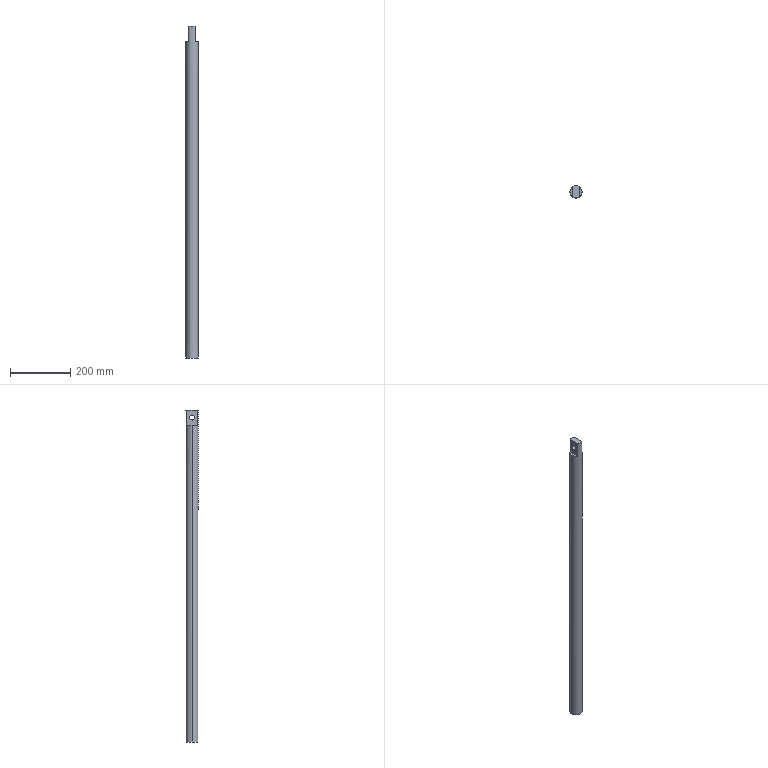Part | SolidWorks | features ICE 2, Extrusion 1 | 1 solid | 10 faces | box 40 x 40 x 1100 mm | volume 1353457 mm3 | plane 6 | cylinder 4 | commonest cylinder face diameters 16.5 x2 40 x2
STEP:
#1=CARTESIAN_POINT('',(10.,0.,1066.75));
#2=VERTEX_POINT('',#1);
#3=CARTESIAN_POINT('',(10.,0.,1083.25));
#4=VERTEX_POINT('',#3);
#5=CARTESIAN_POINT('',(10.,0.,1075.));
#6=DIRECTION('',(-1.,0.,0.));
#7=DIRECTION('',(0.,0.,1.));
#8=AXIS2_PLACEMENT_3D('',#5,#6,#7);
#9=CIRCLE('',#8,8.25);
#10=EDGE_CURVE('',#2,#4,#9,.T.);
#11=ORIENTED_EDGE('',*,*,#10,.F.);
#12=CARTESIAN_POINT('',(-10.,0.,1066.75));
#13=VERTEX_POINT('',#12);
#14=CARTESIAN_POINT('',(20.,0.,1066.75));
#15=DIRECTION('',(-1.,0.,0.));
#16=VECTOR('',#15,1000.);
#17=LINE('',#14,#16);
#18=EDGE_CURVE('',#2,#13,#17,.T.);
#19=ORIENTED_EDGE('',*,*,#18,.T.);
#20=CARTESIAN_POINT('',(-10.,0.,1083.25));
#21=VERTEX_POINT('',#20);
#22=CARTESIAN_POINT('',(-10.,0.,1075.));
#23=DIRECTION('',(1.,0.,0.));
#24=DIRECTION('',(0.,0.,-1.));
#25=AXIS2_PLACEMENT_3D('',#22,#23,#24);
#26=CIRCLE('',#25,8.25);
#27=EDGE_CURVE('',#21,#13,#26,.T.);
#28=ORIENTED_EDGE('',*,*,#27,.F.);
#29=CARTESIAN_POINT('',(20.,0.,1083.25));
#30=DIRECTION('',(-1.,0.,0.));
#31=VECTOR('',#30,1000.);
#32=LINE('',#29,#31);
#33=EDGE_CURVE('',#4,#21,#32,.T.);
#34=ORIENTED_EDGE('',*,*,#33,.F.);
#35=EDGE_LOOP('',(#11,#19,#28,#34));
#36=FACE_OUTER_BOUND('',#35,.T.);
#37=CARTESIAN_POINT('',(20.,0.,1075.));
#38=DIRECTION('',(-1.,0.,0.));
#39=DIRECTION('',(0.,0.,1.));
#40=AXIS2_PLACEMENT_3D('',#37,#38,#39);
#41=CYLINDRICAL_SURFACE('',#40,8.25);
#42=ADVANCED_FACE('',(#36),#41,.F.);
#43=CARTESIAN_POINT('',(10.,17.321,1050.));
#44=VERTEX_POINT('',#43);
#45=CARTESIAN_POINT('',(20.,0.,1050.));
#46=VERTEX_POINT('',#45);
#47=CARTESIAN_POINT('',(0.,0.,1050.));
#48=DIRECTION('',(0.,0.,-1.));
#49=DIRECTION('',(-1.,0.,0.));
#50=AXIS2_PLACEMENT_3D('',#47,#48,#49);
#51=CIRCLE('',#50,20.);
#52=EDGE_CURVE('',#44,#46,#51,.T.);
#53=ORIENTED_EDGE('',*,*,#52,.T.);
#54=CARTESIAN_POINT('',(20.,0.,0.));
#55=VERTEX_POINT('',#54);
#56=CARTESIAN_POINT('',(20.,0.,1100.));
#57=DIRECTION('',(0.,0.,-1.));
#58=VECTOR('',#57,1000.);
#59=LINE('',#56,#58);
#60=EDGE_CURVE('',#46,#55,#59,.T.);
#61=ORIENTED_EDGE('',*,*,#60,.T.);
#62=CARTESIAN_POINT('',(-20.,0.,0.));
#63=VERTEX_POINT('',#62);
#64=CARTESIAN_POINT('',(0.,0.,0.));
#65=DIRECTION('',(0.,0.,1.));
#66=DIRECTION('',(1.,0.,0.));
#67=AXIS2_PLACEMENT_3D('',#64,#65,#66);
#68=CIRCLE('',#67,20.);
#69=EDGE_CURVE('',#55,#63,#68,.T.);
#70=ORIENTED_EDGE('',*,*,#69,.T.);
#71=CARTESIAN_POINT('',(-20.,0.,1050.));
#72=VERTEX_POINT('',#71);
#73=CARTESIAN_POINT('',(-20.,0.,1100.));
#74=DIRECTION('',(0.,0.,-1.));
#75=VECTOR('',#74,1000.);
#76=LINE('',#73,#75);
#77=EDGE_CURVE('',#72,#63,#76,.T.);
#78=ORIENTED_EDGE('',*,*,#77,.F.);
#79=CARTESIAN_POINT('',(-10.,17.321,1050.));
#80=VERTEX_POINT('',#79);
#81=CARTESIAN_POINT('',(0.,0.,1050.));
#82=DIRECTION('',(0.,0.,-1.));
#83=DIRECTION('',(-1.,0.,0.));
#84=AXIS2_PLACEMENT_3D('',#81,#82,#83);
#85=CIRCLE('',#84,20.);
#86=EDGE_CURVE('',#72,#80,#85,.T.);
#87=ORIENTED_EDGE('',*,*,#86,.T.);
#88=CARTESIAN_POINT('',(-10.,17.321,1100.));
#89=VERTEX_POINT('',#88);
#90=CARTESIAN_POINT('',(-10.,17.321,1100.));
#91=DIRECTION('',(0.,0.,1.));
#92=VECTOR('',#91,1000.);
#93=LINE('',#90,#92);
#94=EDGE_CURVE('',#80,#89,#93,.T.);
#95=ORIENTED_EDGE('',*,*,#94,.T.);
#96=CARTESIAN_POINT('',(10.,17.321,1100.));
#97=VERTEX_POINT('',#96);
#98=CARTESIAN_POINT('',(0.,0.,1100.));
#99=DIRECTION('',(0.,0.,1.));
#100=DIRECTION('',(1.,0.,0.));
#101=AXIS2_PLACEMENT_3D('',#98,#99,#100);
#102=CIRCLE('',#101,20.);
#103=EDGE_CURVE('',#97,#89,#102,.T.);
#104=ORIENTED_EDGE('',*,*,#103,.F.);
#105=CARTESIAN_POINT('',(10.,17.321,1100.));
#106=DIRECTION('',(0.,0.,-1.));
#107=VECTOR('',#106,1000.);
#108=LINE('',#105,#107);
#109=EDGE_CURVE('',#97,#44,#108,.T.);
#110=ORIENTED_EDGE('',*,*,#109,.T.);
#111=EDGE_LOOP('',(#53,#61,#70,#78,#87,#95,#104,#110));
#112=FACE_OUTER_BOUND('',#111,.T.);
#113=CARTESIAN_POINT('',(0.,0.,1100.));
#114=DIRECTION('',(0.,0.,-1.));
#115=DIRECTION('',(-1.,0.,0.));
#116=AXIS2_PLACEMENT_3D('',#113,#114,#115);
#117=CYLINDRICAL_SURFACE('',#116,20.);
#118=ADVANCED_FACE('',(#112),#117,.T.);
#119=ORIENTED_EDGE('',*,*,#60,.F.);
#120=CARTESIAN_POINT('',(10.,-17.321,1050.));
#121=VERTEX_POINT('',#120);
#122=CARTESIAN_POINT('',(0.,0.,1050.));
#123=DIRECTION('',(0.,0.,-1.));
#124=DIRECTION('',(-1.,0.,0.));
#125=AXIS2_PLACEMENT_3D('',#122,#123,#124);
#126=CIRCLE('',#125,20.);
#127=EDGE_CURVE('',#46,#121,#126,.T.);
#128=ORIENTED_EDGE('',*,*,#127,.T.);
#129=CARTESIAN_POINT('',(10.,-17.321,1100.));
#130=VERTEX_POINT('',#129);
#131=CARTESIAN_POINT('',(10.,-17.321,1100.));
#132=DIRECTION('',(0.,0.,1.));
#133=VECTOR('',#132,1000.);
#134=LINE('',#131,#133);
#135=EDGE_CURVE('',#121,#130,#134,.T.);
#136=ORIENTED_EDGE('',*,*,#135,.T.);
#137=CARTESIAN_POINT('',(-10.,-17.321,1100.));
#138=VERTEX_POINT('',#137);
#139=CARTESIAN_POINT('',(0.,0.,1100.));
#140=DIRECTION('',(0.,0.,1.));
#141=DIRECTION('',(1.,0.,0.));
#142=AXIS2_PLACEMENT_3D('',#139,#140,#141);
#143=CIRCLE('',#142,20.);
#144=EDGE_CURVE('',#138,#130,#143,.T.);
#145=ORIENTED_EDGE('',*,*,#144,.F.);
#146=CARTESIAN_POINT('',(-10.,-17.321,1050.));
#147=VERTEX_POINT('',#146);
#148=CARTESIAN_POINT('',(-10.,-17.321,1100.));
#149=DIRECTION('',(0.,0.,-1.));
#150=VECTOR('',#149,1000.);
#151=LINE('',#148,#150);
#152=EDGE_CURVE('',#138,#147,#151,.T.);
#153=ORIENTED_EDGE('',*,*,#152,.T.);
#154=CARTESIAN_POINT('',(0.,0.,1050.));
#155=DIRECTION('',(0.,0.,-1.));
#156=DIRECTION('',(-1.,0.,0.));
#157=AXIS2_PLACEMENT_3D('',#154,#155,#156);
#158=CIRCLE('',#157,20.);
#159=EDGE_CURVE('',#147,#72,#158,.T.);
#160=ORIENTED_EDGE('',*,*,#159,.T.);
#161=ORIENTED_EDGE('',*,*,#77,.T.);
#162=CARTESIAN_POINT('',(0.,0.,0.));
#163=DIRECTION('',(0.,0.,1.));
#164=DIRECTION('',(1.,0.,0.));
#165=AXIS2_PLACEMENT_3D('',#162,#163,#164);
#166=CIRCLE('',#165,20.);
#167=EDGE_CURVE('',#63,#55,#166,.T.);
#168=ORIENTED_EDGE('',*,*,#167,.T.);
#169=EDGE_LOOP('',(#119,#128,#136,#145,#153,#160,#161,#168));
#170=FACE_OUTER_BOUND('',#169,.T.);
#171=CARTESIAN_POINT('',(0.,0.,1100.));
#172=DIRECTION('',(0.,0.,-1.));
#173=DIRECTION('',(-1.,0.,0.));
#174=AXIS2_PLACEMENT_3D('',#171,#172,#173);
#175=CYLINDRICAL_SURFACE('',#174,20.);
#176=ADVANCED_FACE('',(#170),#175,.T.);
#177=CARTESIAN_POINT('',(-10.,0.,1100.));
#178=DIRECTION('',(0.,1.,0.));
#179=VECTOR('',#178,1000.);
#180=LINE('',#177,#179);
#181=EDGE_CURVE('',#138,#89,#180,.T.);
#182=ORIENTED_EDGE('',*,*,#181,.F.);
#183=ORIENTED_EDGE('',*,*,#144,.T.);
#184=CARTESIAN_POINT('',(10.,0.,1100.));
#185=DIRECTION('',(0.,-1.,0.));
#186=VECTOR('',#185,1000.);
#187=LINE('',#184,#186);
#188=EDGE_CURVE('',#97,#130,#187,.T.);
#189=ORIENTED_EDGE('',*,*,#188,.F.);
#190=ORIENTED_EDGE('',*,*,#103,.T.);
#191=EDGE_LOOP('',(#182,#183,#189,#190));
#192=FACE_OUTER_BOUND('',#191,.T.);
#193=CARTESIAN_POINT('',(0.,0.,1100.));
#194=DIRECTION('',(0.,0.,1.));
#195=DIRECTION('',(1.,0.,0.));
#196=AXIS2_PLACEMENT_3D('',#193,#194,#195);
#197=PLANE('',#196);
#198=ADVANCED_FACE('',(#192),#197,.T.);
#199=ORIENTED_EDGE('',*,*,#167,.F.);
#200=ORIENTED_EDGE('',*,*,#69,.F.);
#201=EDGE_LOOP('',(#199,#200));
#202=FACE_OUTER_BOUND('',#201,.T.);
#203=CARTESIAN_POINT('',(0.,0.,0.));
#204=DIRECTION('',(0.,0.,1.));
#205=DIRECTION('',(1.,0.,0.));
#206=AXIS2_PLACEMENT_3D('',#203,#204,#205);
#207=PLANE('',#206);
#208=ADVANCED_FACE('',(#202),#207,.F.);
#209=CARTESIAN_POINT('',(10.,-20.,1050.));
#210=DIRECTION('',(0.,1.,0.));
#211=VECTOR('',#210,1000.);
#212=LINE('',#209,#211);
#213=EDGE_CURVE('',#121,#44,#212,.T.);
#214=ORIENTED_EDGE('',*,*,#213,.F.);
#215=ORIENTED_EDGE('',*,*,#127,.F.);
#216=ORIENTED_EDGE('',*,*,#52,.F.);
#217=EDGE_LOOP('',(#214,#215,#216));
#218=FACE_OUTER_BOUND('',#217,.T.);
#219=CARTESIAN_POINT('',(20.,-20.,1050.));
#220=DIRECTION('',(0.,0.,-1.));
#221=DIRECTION('',(-1.,0.,0.));
#222=AXIS2_PLACEMENT_3D('',#219,#220,#221);
#223=PLANE('',#222);
#224=ADVANCED_FACE('',(#218),#223,.F.);
#225=CARTESIAN_POINT('',(10.,0.,1075.));
#226=DIRECTION('',(-1.,0.,0.));
#227=DIRECTION('',(0.,0.,1.));
#228=AXIS2_PLACEMENT_3D('',#225,#226,#227);
#229=CIRCLE('',#228,8.25);
#230=EDGE_CURVE('',#4,#2,#229,.T.);
#231=ORIENTED_EDGE('',*,*,#230,.T.);
#232=ORIENTED_EDGE('',*,*,#10,.T.);
#233=EDGE_LOOP('',(#231,#232));
#234=FACE_BOUND('',#233,.T.);
#235=ORIENTED_EDGE('',*,*,#188,.T.);
#236=ORIENTED_EDGE('',*,*,#135,.F.);
#237=ORIENTED_EDGE('',*,*,#213,.T.);
#238=ORIENTED_EDGE('',*,*,#109,.F.);
#239=EDGE_LOOP('',(#235,#236,#237,#238));
#240=FACE_OUTER_BOUND('',#239,.T.);
#241=CARTESIAN_POINT('',(10.,-20.,1100.));
#242=DIRECTION('',(-1.,0.,0.));
#243=DIRECTION('',(0.,0.,1.));
#244=AXIS2_PLACEMENT_3D('',#241,#242,#243);
#245=PLANE('',#244);
#246=ADVANCED_FACE('',(#234,#240),#245,.F.);
#247=ORIENTED_EDGE('',*,*,#159,.F.);
#248=CARTESIAN_POINT('',(-10.,-20.,1050.));
#249=DIRECTION('',(0.,1.,0.));
#250=VECTOR('',#249,1000.);
#251=LINE('',#248,#250);
#252=EDGE_CURVE('',#147,#80,#251,.T.);
#253=ORIENTED_EDGE('',*,*,#252,.T.);
#254=ORIENTED_EDGE('',*,*,#86,.F.);
#255=EDGE_LOOP('',(#247,#253,#254));
#256=FACE_OUTER_BOUND('',#255,.T.);
#257=CARTESIAN_POINT('',(-20.,-20.,1050.));
#258=DIRECTION('',(0.,0.,-1.));
#259=DIRECTION('',(-1.,0.,0.));
#260=AXIS2_PLACEMENT_3D('',#257,#258,#259);
#261=PLANE('',#260);
#262=ADVANCED_FACE('',(#256),#261,.F.);
#263=ORIENTED_EDGE('',*,*,#27,.T.);
#264=CARTESIAN_POINT('',(-10.,0.,1075.));
#265=DIRECTION('',(1.,0.,0.));
#266=DIRECTION('',(0.,0.,-1.));
#267=AXIS2_PLACEMENT_3D('',#264,#265,#266);
#268=CIRCLE('',#267,8.25);
#269=EDGE_CURVE('',#13,#21,#268,.T.);
#270=ORIENTED_EDGE('',*,*,#269,.T.);
#271=EDGE_LOOP('',(#263,#270));
#272=FACE_BOUND('',#271,.T.);
#273=ORIENTED_EDGE('',*,*,#181,.T.);
#274=ORIENTED_EDGE('',*,*,#94,.F.);
#275=ORIENTED_EDGE('',*,*,#252,.F.);
#276=ORIENTED_EDGE('',*,*,#152,.F.);
#277=EDGE_LOOP('',(#273,#274,#275,#276));
#278=FACE_OUTER_BOUND('',#277,.T.);
#279=CARTESIAN_POINT('',(-10.,-20.,1100.));
#280=DIRECTION('',(1.,0.,0.));
#281=DIRECTION('',(0.,0.,-1.));
#282=AXIS2_PLACEMENT_3D('',#279,#280,#281);
#283=PLANE('',#282);
#284=ADVANCED_FACE('',(#272,#278),#283,.F.);
#285=ORIENTED_EDGE('',*,*,#18,.F.);
#286=ORIENTED_EDGE('',*,*,#230,.F.);
#287=ORIENTED_EDGE('',*,*,#33,.T.);
#288=ORIENTED_EDGE('',*,*,#269,.F.);
#289=EDGE_LOOP('',(#285,#286,#287,#288));
#290=FACE_OUTER_BOUND('',#289,.T.);
#291=CARTESIAN_POINT('',(20.,0.,1075.));
#292=DIRECTION('',(-1.,0.,0.));
#293=DIRECTION('',(0.,0.,1.));
#294=AXIS2_PLACEMENT_3D('',#291,#292,#293);
#295=CYLINDRICAL_SURFACE('',#294,8.25);
#296=ADVANCED_FACE('',(#290),#295,.F.);
#297=CLOSED_SHELL('',(#42,#118,#176,#198,#208,#224,#246,#262,#284,#296));
#298=MANIFOLD_SOLID_BREP('',#297);
#299=CARTESIAN_POINT('',(0.,0.,0.));
#300=DIRECTION('',(0.,0.,1.));
#301=DIRECTION('',(1.,0.,0.));
#302=AXIS2_PLACEMENT_3D('',#299,#300,#301);
#303=(LENGTH_UNIT()NAMED_UNIT(*)SI_UNIT(.MILLI.,.METRE.));
#304=UNCERTAINTY_MEASURE_WITH_UNIT(LENGTH_MEASURE(0.00001),#303,'','');
#305=(NAMED_UNIT(*)PLANE_ANGLE_UNIT()SI_UNIT($,.RADIAN.));
#306=(NAMED_UNIT(*)SI_UNIT($,.STERADIAN.)SOLID_ANGLE_UNIT());
#307=(GEOMETRIC_REPRESENTATION_CONTEXT(3)GLOBAL_UNCERTAINTY_ASSIGNED_CONTEXT((#304))GLOBAL_UNIT_ASSIGNED_CONTEXT((#303,#305,#306))REPRESENTATION_CONTEXT('',''));
#308=ADVANCED_BREP_SHAPE_REPRESENTATION('',(#298,#302),#307);